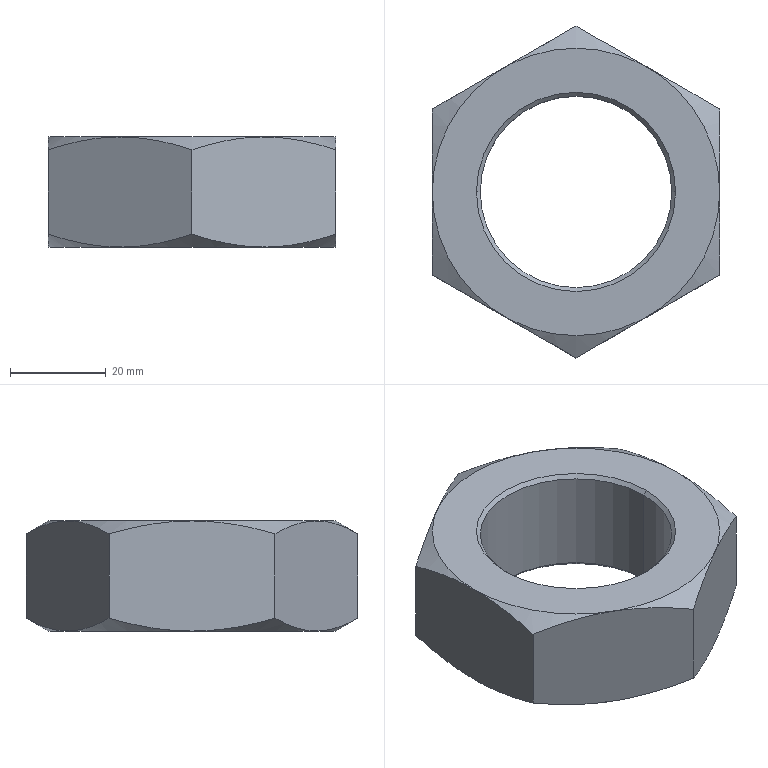Part | STEP file | NT-18_Nuts | 1 solid | 18 faces | box 60.016 x 69.3 x 23 mm | volume 42288 mm3 | cone 8 | plane 8 | cylinder 2 | commonest cylinder face diameters 40 x2